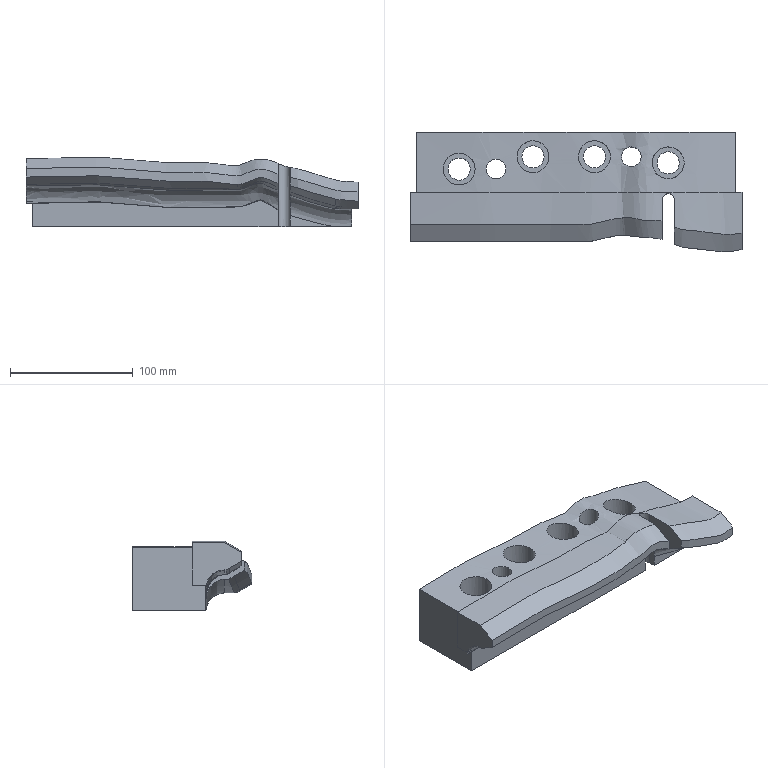Part | NX | features solid 2 | 1 solid | 53 faces | box 270 x 97.367 x 56.346 mm | volume 794405 mm3 | spline 22 | plane 20 | cylinder 11 | commonest cylinder face diameters 18 x4 26 x4 16 x2 10 x1